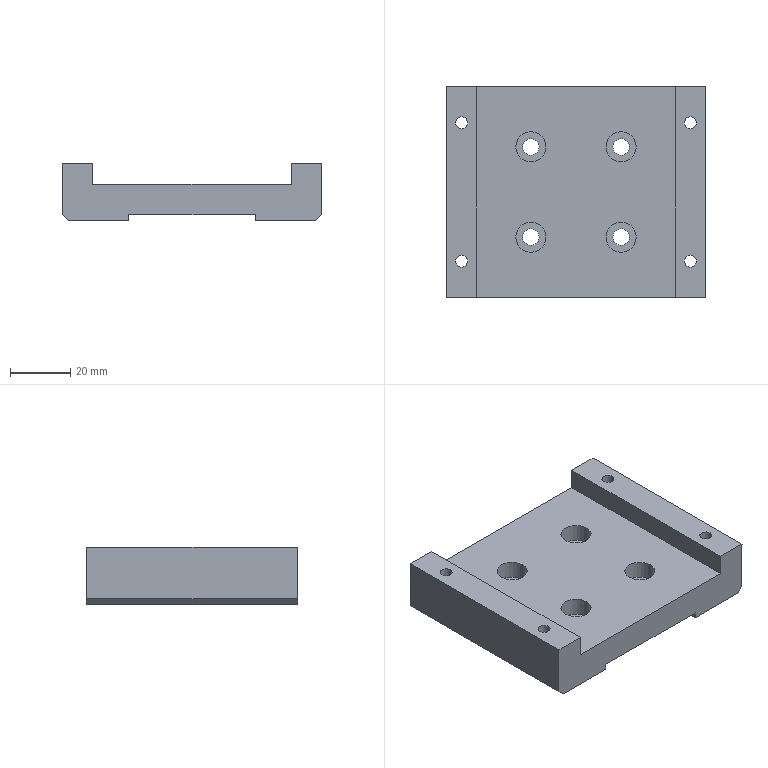Part | STEP file | ASND-0110-LPMF01-034 | 1 solid | 52 faces | box 86 x 70 x 19 mm | volume 72514 mm3 | cylinder 28 | plane 20 | cone 4 | commonest cylinder face diameters 4 x8 5.5 x8 10 x8 2 x4